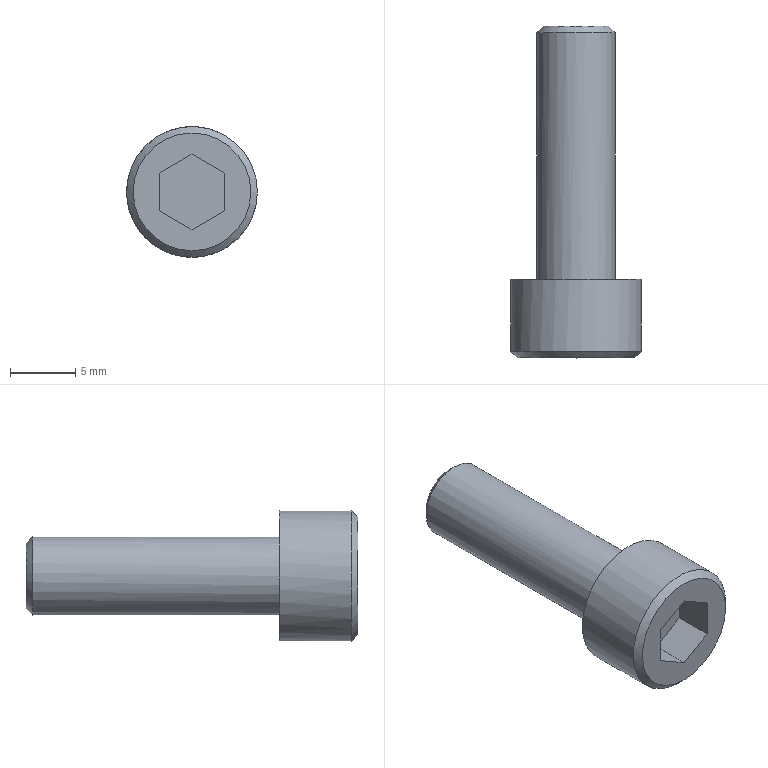Part | NX | features M6.00-40.00 2 | 1 solid | 14 faces | box 10 x 25.368 x 10 mm | volume 947.893 mm3 | plane 10 | cylinder 2 | cone 2 | commonest cylinder face diameters 6 x1 10 x1
STEP:
#1=CARTESIAN_POINT('',(0.,-145.368,21.225));
#2=VERTEX_POINT('',#1);
#3=CARTESIAN_POINT('',(0.,-145.368,25.725));
#4=DIRECTION('',(0.,-1.,0.));
#5=DIRECTION('',(0.,0.,-1.));
#6=AXIS2_PLACEMENT_3D('',#3,#4,#5);
#7=CIRCLE('',#6,4.5);
#8=EDGE_CURVE('',#2,#2,#7,.T.);
#9=ORIENTED_EDGE('',*,*,#8,.T.);
#10=EDGE_LOOP('',(#9));
#11=FACE_BOUND('',#10,.T.);
#12=CARTESIAN_POINT('',(-2.5,-145.368,27.169));
#13=VERTEX_POINT('',#12);
#14=CARTESIAN_POINT('',(-2.5,-145.368,24.282));
#15=VERTEX_POINT('',#14);
#16=CARTESIAN_POINT('',(-2.5,-145.368,27.169));
#17=DIRECTION('',(0.,0.,-1.));
#18=VECTOR('',#17,1000.);
#19=LINE('',#16,#18);
#20=EDGE_CURVE('',#13,#15,#19,.T.);
#21=ORIENTED_EDGE('',*,*,#20,.F.);
#22=CARTESIAN_POINT('',(0.,-145.368,28.612));
#23=VERTEX_POINT('',#22);
#24=CARTESIAN_POINT('',(0.,-145.368,28.612));
#25=DIRECTION('',(-0.866,0.,-0.5));
#26=VECTOR('',#25,1000.);
#27=LINE('',#24,#26);
#28=EDGE_CURVE('',#23,#13,#27,.T.);
#29=ORIENTED_EDGE('',*,*,#28,.F.);
#30=CARTESIAN_POINT('',(2.5,-145.368,27.169));
#31=VERTEX_POINT('',#30);
#32=CARTESIAN_POINT('',(2.5,-145.368,27.169));
#33=DIRECTION('',(-0.866,0.,0.5));
#34=VECTOR('',#33,1000.);
#35=LINE('',#32,#34);
#36=EDGE_CURVE('',#31,#23,#35,.T.);
#37=ORIENTED_EDGE('',*,*,#36,.F.);
#38=CARTESIAN_POINT('',(2.5,-145.368,24.282));
#39=VERTEX_POINT('',#38);
#40=CARTESIAN_POINT('',(2.5,-145.368,24.282));
#41=DIRECTION('',(0.,0.,1.));
#42=VECTOR('',#41,1000.);
#43=LINE('',#40,#42);
#44=EDGE_CURVE('',#39,#31,#43,.T.);
#45=ORIENTED_EDGE('',*,*,#44,.F.);
#46=CARTESIAN_POINT('',(0.,-145.368,22.838));
#47=VERTEX_POINT('',#46);
#48=CARTESIAN_POINT('',(0.,-145.368,22.838));
#49=DIRECTION('',(0.866,0.,0.5));
#50=VECTOR('',#49,1000.);
#51=LINE('',#48,#50);
#52=EDGE_CURVE('',#47,#39,#51,.T.);
#53=ORIENTED_EDGE('',*,*,#52,.F.);
#54=CARTESIAN_POINT('',(-2.5,-145.368,24.282));
#55=DIRECTION('',(0.866,0.,-0.5));
#56=VECTOR('',#55,1000.);
#57=LINE('',#54,#56);
#58=EDGE_CURVE('',#15,#47,#57,.T.);
#59=ORIENTED_EDGE('',*,*,#58,.F.);
#60=EDGE_LOOP('',(#21,#29,#37,#45,#53,#59));
#61=FACE_BOUND('',#60,.T.);
#62=CARTESIAN_POINT('',(0.,-145.368,25.725));
#63=DIRECTION('',(0.,-1.,0.));
#64=DIRECTION('',(0.,0.,-1.));
#65=AXIS2_PLACEMENT_3D('',#62,#63,#64);
#66=PLANE('',#65);
#67=ADVANCED_FACE('',(#11,#61),#66,.T.);
#68=CARTESIAN_POINT('',(3.,-139.368,25.725));
#69=VERTEX_POINT('',#68);
#70=CARTESIAN_POINT('',(0.,-139.368,25.725));
#71=DIRECTION('',(0.,1.,0.));
#72=DIRECTION('',(1.,0.,0.));
#73=AXIS2_PLACEMENT_3D('',#70,#71,#72);
#74=CIRCLE('',#73,3.);
#75=EDGE_CURVE('',#69,#69,#74,.T.);
#76=ORIENTED_EDGE('',*,*,#75,.F.);
#77=EDGE_LOOP('',(#76));
#78=FACE_BOUND('',#77,.T.);
#79=CARTESIAN_POINT('',(5.,-139.368,25.725));
#80=VERTEX_POINT('',#79);
#81=CARTESIAN_POINT('',(0.,-139.368,25.725));
#82=DIRECTION('',(0.,-1.,0.));
#83=DIRECTION('',(1.,0.,0.));
#84=AXIS2_PLACEMENT_3D('',#81,#82,#83);
#85=CIRCLE('',#84,5.);
#86=EDGE_CURVE('',#80,#80,#85,.T.);
#87=ORIENTED_EDGE('',*,*,#86,.F.);
#88=EDGE_LOOP('',(#87));
#89=FACE_BOUND('',#88,.T.);
#90=CARTESIAN_POINT('',(0.,-139.368,25.725));
#91=DIRECTION('',(0.,1.,0.));
#92=DIRECTION('',(0.,0.,1.));
#93=AXIS2_PLACEMENT_3D('',#90,#91,#92);
#94=PLANE('',#93);
#95=ADVANCED_FACE('',(#78,#89),#94,.T.);
#96=CARTESIAN_POINT('',(0.,-144.868,20.725));
#97=VERTEX_POINT('',#96);
#98=CARTESIAN_POINT('',(0.,-144.868,25.725));
#99=DIRECTION('',(0.,-1.,0.));
#100=DIRECTION('',(0.,0.,-1.));
#101=AXIS2_PLACEMENT_3D('',#98,#99,#100);
#102=CIRCLE('',#101,5.);
#103=EDGE_CURVE('',#97,#97,#102,.F.);
#104=ORIENTED_EDGE('',*,*,#103,.T.);
#105=EDGE_LOOP('',(#104));
#106=FACE_BOUND('',#105,.T.);
#107=ORIENTED_EDGE('',*,*,#86,.T.);
#108=EDGE_LOOP('',(#107));
#109=FACE_BOUND('',#108,.T.);
#110=CARTESIAN_POINT('',(0.,-139.368,25.725));
#111=DIRECTION('',(0.,-1.,0.));
#112=DIRECTION('',(1.,0.,0.));
#113=AXIS2_PLACEMENT_3D('',#110,#111,#112);
#114=CYLINDRICAL_SURFACE('',#113,5.);
#115=ADVANCED_FACE('',(#106,#109),#114,.T.);
#116=CARTESIAN_POINT('',(0.,-120.,28.225));
#117=VERTEX_POINT('',#116);
#118=CARTESIAN_POINT('',(0.,-120.,25.725));
#119=DIRECTION('',(0.,1.,0.));
#120=DIRECTION('',(0.,0.,1.));
#121=AXIS2_PLACEMENT_3D('',#118,#119,#120);
#122=CIRCLE('',#121,2.5);
#123=EDGE_CURVE('',#117,#117,#122,.T.);
#124=ORIENTED_EDGE('',*,*,#123,.T.);
#125=EDGE_LOOP('',(#124));
#126=FACE_BOUND('',#125,.T.);
#127=CARTESIAN_POINT('',(0.,-120.,25.725));
#128=DIRECTION('',(0.,1.,0.));
#129=DIRECTION('',(0.,0.,1.));
#130=AXIS2_PLACEMENT_3D('',#127,#128,#129);
#131=PLANE('',#130);
#132=ADVANCED_FACE('',(#126),#131,.T.);
#133=CARTESIAN_POINT('',(0.,-120.5,28.725));
#134=VERTEX_POINT('',#133);
#135=CARTESIAN_POINT('',(0.,-120.5,25.725));
#136=DIRECTION('',(0.,1.,0.));
#137=DIRECTION('',(0.,0.,1.));
#138=AXIS2_PLACEMENT_3D('',#135,#136,#137);
#139=CIRCLE('',#138,3.);
#140=EDGE_CURVE('',#134,#134,#139,.F.);
#141=ORIENTED_EDGE('',*,*,#140,.T.);
#142=EDGE_LOOP('',(#141));
#143=FACE_BOUND('',#142,.T.);
#144=ORIENTED_EDGE('',*,*,#75,.T.);
#145=EDGE_LOOP('',(#144));
#146=FACE_BOUND('',#145,.T.);
#147=CARTESIAN_POINT('',(0.,-151.368,25.725));
#148=DIRECTION('',(0.,1.,0.));
#149=DIRECTION('',(1.,0.,0.));
#150=AXIS2_PLACEMENT_3D('',#147,#148,#149);
#151=CYLINDRICAL_SURFACE('',#150,3.);
#152=ADVANCED_FACE('',(#143,#146),#151,.T.);
#153=ORIENTED_EDGE('',*,*,#58,.T.);
#154=CARTESIAN_POINT('',(0.,-142.368,22.838));
#155=VERTEX_POINT('',#154);
#156=CARTESIAN_POINT('',(0.,-142.368,22.838));
#157=DIRECTION('',(0.,-1.,0.));
#158=VECTOR('',#157,1000.);
#159=LINE('',#156,#158);
#160=EDGE_CURVE('',#47,#155,#159,.F.);
#161=ORIENTED_EDGE('',*,*,#160,.T.);
#162=CARTESIAN_POINT('',(-2.5,-142.368,24.282));
#163=VERTEX_POINT('',#162);
#164=CARTESIAN_POINT('',(-2.5,-142.368,24.282));
#165=DIRECTION('',(0.866,0.,-0.5));
#166=VECTOR('',#165,1000.);
#167=LINE('',#164,#166);
#168=EDGE_CURVE('',#155,#163,#167,.F.);
#169=ORIENTED_EDGE('',*,*,#168,.T.);
#170=CARTESIAN_POINT('',(-2.5,-142.368,24.282));
#171=DIRECTION('',(0.,-1.,0.));
#172=VECTOR('',#171,1000.);
#173=LINE('',#170,#172);
#174=EDGE_CURVE('',#15,#163,#173,.F.);
#175=ORIENTED_EDGE('',*,*,#174,.F.);
#176=EDGE_LOOP('',(#153,#161,#169,#175));
#177=FACE_BOUND('',#176,.T.);
#178=CARTESIAN_POINT('',(-1.25,-143.868,23.56));
#179=DIRECTION('',(-0.5,0.,-0.866));
#180=DIRECTION('',(-0.866,0.,0.5));
#181=AXIS2_PLACEMENT_3D('',#178,#179,#180);
#182=PLANE('',#181);
#183=ADVANCED_FACE('',(#177),#182,.F.);
#184=ORIENTED_EDGE('',*,*,#20,.T.);
#185=ORIENTED_EDGE('',*,*,#174,.T.);
#186=CARTESIAN_POINT('',(-2.5,-142.368,27.169));
#187=VERTEX_POINT('',#186);
#188=CARTESIAN_POINT('',(-2.5,-142.368,27.169));
#189=DIRECTION('',(0.,0.,-1.));
#190=VECTOR('',#189,1000.);
#191=LINE('',#188,#190);
#192=EDGE_CURVE('',#163,#187,#191,.F.);
#193=ORIENTED_EDGE('',*,*,#192,.T.);
#194=CARTESIAN_POINT('',(-2.5,-142.368,27.169));
#195=DIRECTION('',(0.,-1.,0.));
#196=VECTOR('',#195,1000.);
#197=LINE('',#194,#196);
#198=EDGE_CURVE('',#13,#187,#197,.F.);
#199=ORIENTED_EDGE('',*,*,#198,.F.);
#200=EDGE_LOOP('',(#184,#185,#193,#199));
#201=FACE_BOUND('',#200,.T.);
#202=CARTESIAN_POINT('',(-2.5,-143.868,25.725));
#203=DIRECTION('',(-1.,0.,0.));
#204=DIRECTION('',(0.,-1.,0.));
#205=AXIS2_PLACEMENT_3D('',#202,#203,#204);
#206=PLANE('',#205);
#207=ADVANCED_FACE('',(#201),#206,.F.);
#208=ORIENTED_EDGE('',*,*,#28,.T.);
#209=ORIENTED_EDGE('',*,*,#198,.T.);
#210=CARTESIAN_POINT('',(0.,-142.368,28.612));
#211=VERTEX_POINT('',#210);
#212=CARTESIAN_POINT('',(0.,-142.368,28.612));
#213=DIRECTION('',(-0.866,0.,-0.5));
#214=VECTOR('',#213,1000.);
#215=LINE('',#212,#214);
#216=EDGE_CURVE('',#187,#211,#215,.F.);
#217=ORIENTED_EDGE('',*,*,#216,.T.);
#218=CARTESIAN_POINT('',(0.,-142.368,28.612));
#219=DIRECTION('',(0.,-1.,0.));
#220=VECTOR('',#219,1000.);
#221=LINE('',#218,#220);
#222=EDGE_CURVE('',#23,#211,#221,.F.);
#223=ORIENTED_EDGE('',*,*,#222,.F.);
#224=EDGE_LOOP('',(#208,#209,#217,#223));
#225=FACE_BOUND('',#224,.T.);
#226=CARTESIAN_POINT('',(-1.25,-143.868,27.89));
#227=DIRECTION('',(-0.5,0.,0.866));
#228=DIRECTION('',(0.866,0.,0.5));
#229=AXIS2_PLACEMENT_3D('',#226,#227,#228);
#230=PLANE('',#229);
#231=ADVANCED_FACE('',(#225),#230,.F.);
#232=ORIENTED_EDGE('',*,*,#36,.T.);
#233=ORIENTED_EDGE('',*,*,#222,.T.);
#234=CARTESIAN_POINT('',(2.5,-142.368,27.169));
#235=VERTEX_POINT('',#234);
#236=CARTESIAN_POINT('',(2.5,-142.368,27.169));
#237=DIRECTION('',(-0.866,0.,0.5));
#238=VECTOR('',#237,1000.);
#239=LINE('',#236,#238);
#240=EDGE_CURVE('',#211,#235,#239,.F.);
#241=ORIENTED_EDGE('',*,*,#240,.T.);
#242=CARTESIAN_POINT('',(2.5,-142.368,27.169));
#243=DIRECTION('',(0.,-1.,0.));
#244=VECTOR('',#243,1000.);
#245=LINE('',#242,#244);
#246=EDGE_CURVE('',#31,#235,#245,.F.);
#247=ORIENTED_EDGE('',*,*,#246,.F.);
#248=EDGE_LOOP('',(#232,#233,#241,#247));
#249=FACE_BOUND('',#248,.T.);
#250=CARTESIAN_POINT('',(1.25,-143.868,27.89));
#251=DIRECTION('',(0.5,0.,0.866));
#252=DIRECTION('',(0.866,0.,-0.5));
#253=AXIS2_PLACEMENT_3D('',#250,#251,#252);
#254=PLANE('',#253);
#255=ADVANCED_FACE('',(#249),#254,.F.);
#256=ORIENTED_EDGE('',*,*,#44,.T.);
#257=ORIENTED_EDGE('',*,*,#246,.T.);
#258=CARTESIAN_POINT('',(2.5,-142.368,24.282));
#259=VERTEX_POINT('',#258);
#260=CARTESIAN_POINT('',(2.5,-142.368,24.282));
#261=DIRECTION('',(0.,0.,1.));
#262=VECTOR('',#261,1000.);
#263=LINE('',#260,#262);
#264=EDGE_CURVE('',#235,#259,#263,.F.);
#265=ORIENTED_EDGE('',*,*,#264,.T.);
#266=CARTESIAN_POINT('',(2.5,-142.368,24.282));
#267=DIRECTION('',(0.,-1.,0.));
#268=VECTOR('',#267,1000.);
#269=LINE('',#266,#268);
#270=EDGE_CURVE('',#39,#259,#269,.F.);
#271=ORIENTED_EDGE('',*,*,#270,.F.);
#272=EDGE_LOOP('',(#256,#257,#265,#271));
#273=FACE_BOUND('',#272,.T.);
#274=CARTESIAN_POINT('',(2.5,-143.868,25.725));
#275=DIRECTION('',(1.,0.,0.));
#276=DIRECTION('',(0.,0.,-1.));
#277=AXIS2_PLACEMENT_3D('',#274,#275,#276);
#278=PLANE('',#277);
#279=ADVANCED_FACE('',(#273),#278,.F.);
#280=ORIENTED_EDGE('',*,*,#52,.T.);
#281=ORIENTED_EDGE('',*,*,#270,.T.);
#282=CARTESIAN_POINT('',(0.,-142.368,22.838));
#283=DIRECTION('',(0.866,0.,0.5));
#284=VECTOR('',#283,1000.);
#285=LINE('',#282,#284);
#286=EDGE_CURVE('',#259,#155,#285,.F.);
#287=ORIENTED_EDGE('',*,*,#286,.T.);
#288=ORIENTED_EDGE('',*,*,#160,.F.);
#289=EDGE_LOOP('',(#280,#281,#287,#288));
#290=FACE_BOUND('',#289,.T.);
#291=CARTESIAN_POINT('',(1.25,-143.868,23.56));
#292=DIRECTION('',(0.5,0.,-0.866));
#293=DIRECTION('',(-0.866,0.,-0.5));
#294=AXIS2_PLACEMENT_3D('',#291,#292,#293);
#295=PLANE('',#294);
#296=ADVANCED_FACE('',(#290),#295,.F.);
#297=ORIENTED_EDGE('',*,*,#286,.F.);
#298=ORIENTED_EDGE('',*,*,#264,.F.);
#299=ORIENTED_EDGE('',*,*,#240,.F.);
#300=ORIENTED_EDGE('',*,*,#216,.F.);
#301=ORIENTED_EDGE('',*,*,#192,.F.);
#302=ORIENTED_EDGE('',*,*,#168,.F.);
#303=EDGE_LOOP('',(#297,#298,#299,#300,#301,#302));
#304=FACE_BOUND('',#303,.T.);
#305=CARTESIAN_POINT('',(0.,-142.368,25.725));
#306=DIRECTION('',(0.,1.,0.));
#307=DIRECTION('',(0.,0.,1.));
#308=AXIS2_PLACEMENT_3D('',#305,#306,#307);
#309=PLANE('',#308);
#310=ADVANCED_FACE('',(#304),#309,.F.);
#311=ORIENTED_EDGE('',*,*,#123,.F.);
#312=EDGE_LOOP('',(#311));
#313=FACE_BOUND('',#312,.T.);
#314=ORIENTED_EDGE('',*,*,#140,.F.);
#315=EDGE_LOOP('',(#314));
#316=FACE_BOUND('',#315,.T.);
#317=CARTESIAN_POINT('',(0.,-120.5,25.725));
#318=DIRECTION('',(0.,-1.,0.));
#319=DIRECTION('',(0.,0.,-1.));
#320=AXIS2_PLACEMENT_3D('',#317,#318,#319);
#321=CONICAL_SURFACE('',#320,3.,0.7854);
#322=ADVANCED_FACE('',(#313,#316),#321,.T.);
#323=ORIENTED_EDGE('',*,*,#8,.F.);
#324=EDGE_LOOP('',(#323));
#325=FACE_BOUND('',#324,.T.);
#326=ORIENTED_EDGE('',*,*,#103,.F.);
#327=EDGE_LOOP('',(#326));
#328=FACE_BOUND('',#327,.T.);
#329=CARTESIAN_POINT('',(0.,-144.868,25.725));
#330=DIRECTION('',(0.,1.,0.));
#331=DIRECTION('',(0.,0.,1.));
#332=AXIS2_PLACEMENT_3D('',#329,#330,#331);
#333=CONICAL_SURFACE('',#332,5.,0.7854);
#334=ADVANCED_FACE('',(#325,#328),#333,.T.);
#335=CLOSED_SHELL('',(#67,#95,#115,#132,#152,#183,#207,#231,#255,#279,#296,#310,#322,#334));
#336=MANIFOLD_SOLID_BREP('',#335);
#337=(LENGTH_UNIT()NAMED_UNIT(*)SI_UNIT(.MILLI.,.METRE.));
#338=UNCERTAINTY_MEASURE_WITH_UNIT(LENGTH_MEASURE(0.00001),#337,'','');
#339=(NAMED_UNIT(*)PLANE_ANGLE_UNIT()SI_UNIT($,.RADIAN.));
#340=(NAMED_UNIT(*)SI_UNIT($,.STERADIAN.)SOLID_ANGLE_UNIT());
#341=(GEOMETRIC_REPRESENTATION_CONTEXT(3)GLOBAL_UNCERTAINTY_ASSIGNED_CONTEXT((#338))GLOBAL_UNIT_ASSIGNED_CONTEXT((#337,#339,#340))REPRESENTATION_CONTEXT('',''));
#342=ADVANCED_BREP_SHAPE_REPRESENTATION('',(#336),#341);